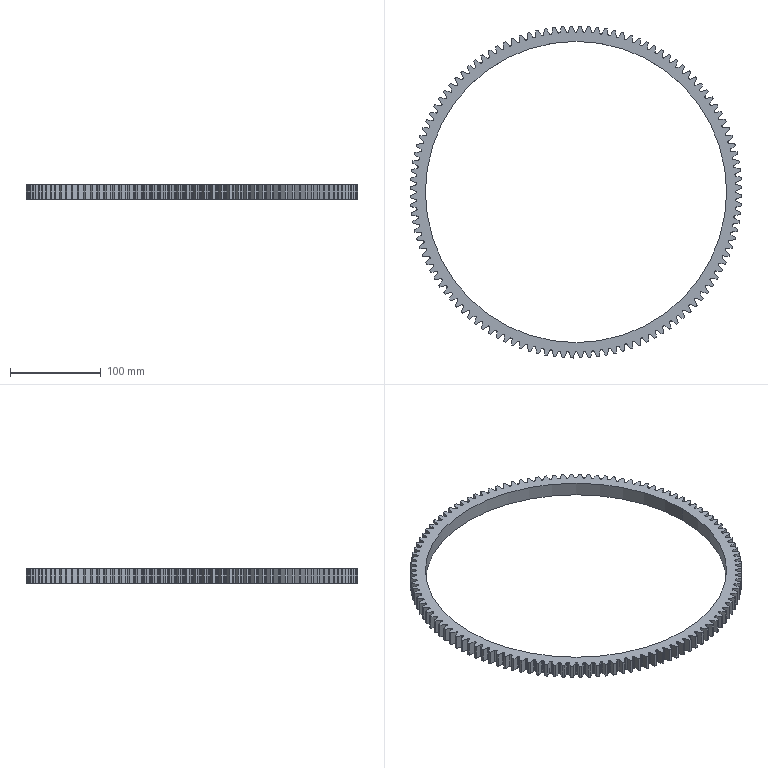Part | SolidWorks | features BaseBody 1 | 1 solid | 774 faces | box 365.943 x 365.943 x 15.5 mm | volume 232827 mm3 | cylinder 532 | spline 240 | plane 2 | commonest cylinder face diameters 2.28 x290 352.5 x120 366 x120 332 x2